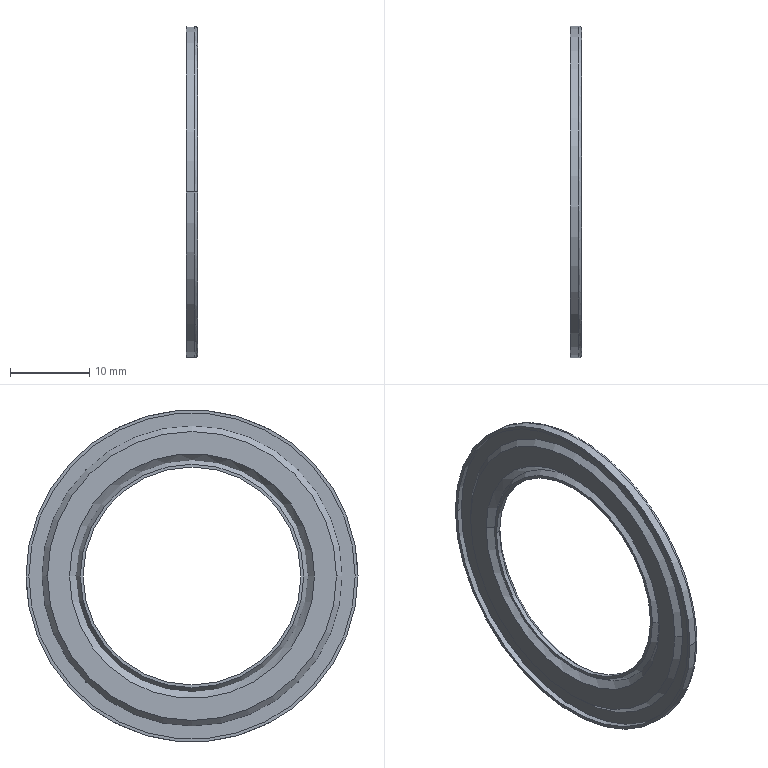Part | STEP file | Microwave Drying Flat Conveyor-inafag_ucfl204_62o9y6gnj3059x015y4y3bh4_09 | 1 solid | 27 faces | box 1.397 x 42 x 42 mm | volume 599.533 mm3 | cone 12 | plane 7 | cylinder 6 | spline 2 | commonest cylinder face diameters 27.56 x2 41.278 x2 42 x2
STEP:
#1=CARTESIAN_POINT('',(8.679,21.,0.));
#2=VERTEX_POINT('',#1);
#3=CARTESIAN_POINT('',(8.679,-21.,0.));
#4=VERTEX_POINT('',#3);
#5=CARTESIAN_POINT('',(8.679,0.,0.));
#6=DIRECTION('',(-1.,0.,0.));
#7=DIRECTION('',(0.,-1.,0.));
#8=AXIS2_PLACEMENT_3D('',#5,#6,#7);
#9=CIRCLE('',#8,21.);
#10=EDGE_CURVE('',#2,#4,#9,.T.);
#11=ORIENTED_EDGE('',*,*,#10,.F.);
#12=CARTESIAN_POINT('',(9.04,20.639,0.));
#13=VERTEX_POINT('',#12);
#14=CARTESIAN_POINT('',(8.679,20.639,0.));
#15=DIRECTION('',(0.,0.,-1.));
#16=DIRECTION('',(0.,1.,0.));
#17=AXIS2_PLACEMENT_3D('',#14,#15,#16);
#18=CIRCLE('',#17,0.361);
#19=EDGE_CURVE('',#2,#13,#18,.T.);
#20=ORIENTED_EDGE('',*,*,#19,.T.);
#21=CARTESIAN_POINT('',(9.04,-20.639,0.));
#22=VERTEX_POINT('',#21);
#23=CARTESIAN_POINT('',(9.04,20.639,0.));
#24=CARTESIAN_POINT('',(9.04,20.639,-41.278));
#25=CARTESIAN_POINT('',(9.04,-20.639,-41.278));
#26=CARTESIAN_POINT('',(9.04,-20.639,0.));
#27=(BOUNDED_CURVE()B_SPLINE_CURVE(3,(#23,#24,#25,#26),.UNSPECIFIED.,.F.,.F.)B_SPLINE_CURVE_WITH_KNOTS((4,4),(0.25,0.75),.UNSPECIFIED.)CURVE()GEOMETRIC_REPRESENTATION_ITEM()RATIONAL_B_SPLINE_CURVE((1.,0.3333,0.3333,1.))REPRESENTATION_ITEM(''));
#28=EDGE_CURVE('',#13,#22,#27,.T.);
#29=ORIENTED_EDGE('',*,*,#28,.T.);
#30=CARTESIAN_POINT('',(8.679,-20.639,0.));
#31=DIRECTION('',(0.,0.,1.));
#32=DIRECTION('',(0.,-1.,0.));
#33=AXIS2_PLACEMENT_3D('',#30,#31,#32);
#34=CIRCLE('',#33,0.361);
#35=EDGE_CURVE('',#4,#22,#34,.T.);
#36=ORIENTED_EDGE('',*,*,#35,.F.);
#37=EDGE_LOOP('',(#11,#20,#29,#36));
#38=FACE_OUTER_BOUND('',#37,.T.);
#39=CARTESIAN_POINT('',(8.679,21.,0.));
#40=CARTESIAN_POINT('',(8.679,21.,-42.));
#41=CARTESIAN_POINT('',(8.679,-21.,-42.));
#42=CARTESIAN_POINT('',(8.679,-21.,0.));
#43=CARTESIAN_POINT('',(8.89,21.,0.));
#44=CARTESIAN_POINT('',(8.89,21.,-42.));
#45=CARTESIAN_POINT('',(8.89,-21.,-42.));
#46=CARTESIAN_POINT('',(8.89,-21.,0.));
#47=CARTESIAN_POINT('',(9.04,20.85,0.));
#48=CARTESIAN_POINT('',(9.04,20.85,-41.701));
#49=CARTESIAN_POINT('',(9.04,-20.85,-41.701));
#50=CARTESIAN_POINT('',(9.04,-20.85,0.));
#51=CARTESIAN_POINT('',(9.04,20.639,0.));
#52=CARTESIAN_POINT('',(9.04,20.639,-41.278));
#53=CARTESIAN_POINT('',(9.04,-20.639,-41.278));
#54=CARTESIAN_POINT('',(9.04,-20.639,0.));
#55=(BOUNDED_SURFACE()B_SPLINE_SURFACE(3,3,((#39,#40,#41,#42),(#43,#44,#45,#46),(#47,#48,#49,#50),(#51,#52,#53,#54)),.UNSPECIFIED.,.F.,.F.,.F.)B_SPLINE_SURFACE_WITH_KNOTS((4,4),(4,4),(0.,1.),(0.,1.),.UNSPECIFIED.)GEOMETRIC_REPRESENTATION_ITEM()RATIONAL_B_SPLINE_SURFACE(((1.,0.3333,0.3333,1.),(0.8047,0.2682,0.2682,0.8047),(0.8047,0.2682,0.2682,0.8047),(1.,0.3333,0.3333,1.)))REPRESENTATION_ITEM('')SURFACE());
#56=ADVANCED_FACE('',(#38),#55,.T.);
#57=CARTESIAN_POINT('',(7.643,-18.275,0.));
#58=VERTEX_POINT('',#57);
#59=CARTESIAN_POINT('',(7.643,18.275,0.));
#60=VERTEX_POINT('',#59);
#61=CARTESIAN_POINT('',(7.643,0.,0.));
#62=DIRECTION('',(-1.,0.,0.));
#63=DIRECTION('',(0.,1.,0.));
#64=AXIS2_PLACEMENT_3D('',#61,#62,#63);
#65=CIRCLE('',#64,18.275);
#66=EDGE_CURVE('',#58,#60,#65,.T.);
#67=ORIENTED_EDGE('',*,*,#66,.F.);
#68=CARTESIAN_POINT('',(8.341,-18.974,0.));
#69=VERTEX_POINT('',#68);
#70=CARTESIAN_POINT('',(8.342,-18.974,0.));
#71=DIRECTION('',(0.7071,-0.7071,0.));
#72=VECTOR('',#71,1000.);
#73=LINE('',#70,#72);
#74=EDGE_CURVE('',#58,#69,#73,.T.);
#75=ORIENTED_EDGE('',*,*,#74,.T.);
#76=CARTESIAN_POINT('',(8.342,18.974,0.));
#77=VERTEX_POINT('',#76);
#78=CARTESIAN_POINT('',(8.342,0.,0.));
#79=DIRECTION('',(-1.,0.,0.));
#80=DIRECTION('',(0.,1.,0.));
#81=AXIS2_PLACEMENT_3D('',#78,#79,#80);
#82=CIRCLE('',#81,18.974);
#83=EDGE_CURVE('',#69,#77,#82,.T.);
#84=ORIENTED_EDGE('',*,*,#83,.T.);
#85=CARTESIAN_POINT('',(8.342,18.974,0.));
#86=DIRECTION('',(0.7071,0.7071,0.));
#87=VECTOR('',#86,1000.);
#88=LINE('',#85,#87);
#89=EDGE_CURVE('',#60,#77,#88,.T.);
#90=ORIENTED_EDGE('',*,*,#89,.F.);
#91=EDGE_LOOP('',(#67,#75,#84,#90));
#92=FACE_OUTER_BOUND('',#91,.T.);
#93=CARTESIAN_POINT('',(8.342,0.,0.));
#94=DIRECTION('',(1.,0.,0.));
#95=DIRECTION('',(0.,1.,0.));
#96=AXIS2_PLACEMENT_3D('',#93,#94,#95);
#97=CONICAL_SURFACE('',#96,18.974,0.7854);
#98=ADVANCED_FACE('',(#92),#97,.T.);
#99=CARTESIAN_POINT('',(8.481,-14.659,0.));
#100=VERTEX_POINT('',#99);
#101=CARTESIAN_POINT('',(8.481,14.659,0.));
#102=VERTEX_POINT('',#101);
#103=CARTESIAN_POINT('',(8.481,0.,0.));
#104=DIRECTION('',(1.,0.,0.));
#105=DIRECTION('',(0.,0.,1.));
#106=AXIS2_PLACEMENT_3D('',#103,#104,#105);
#107=CIRCLE('',#106,14.659);
#108=EDGE_CURVE('',#100,#102,#107,.T.);
#109=ORIENTED_EDGE('',*,*,#108,.T.);
#110=CARTESIAN_POINT('',(7.643,15.497,0.));
#111=VERTEX_POINT('',#110);
#112=CARTESIAN_POINT('',(8.481,14.659,0.));
#113=DIRECTION('',(-0.7071,0.7071,0.));
#114=VECTOR('',#113,1000.);
#115=LINE('',#112,#114);
#116=EDGE_CURVE('',#102,#111,#115,.T.);
#117=ORIENTED_EDGE('',*,*,#116,.T.);
#118=CARTESIAN_POINT('',(7.643,-15.497,0.));
#119=VERTEX_POINT('',#118);
#120=CARTESIAN_POINT('',(7.643,0.,0.));
#121=DIRECTION('',(1.,0.,0.));
#122=DIRECTION('',(0.,-1.,0.));
#123=AXIS2_PLACEMENT_3D('',#120,#121,#122);
#124=CIRCLE('',#123,15.497);
#125=EDGE_CURVE('',#119,#111,#124,.T.);
#126=ORIENTED_EDGE('',*,*,#125,.F.);
#127=CARTESIAN_POINT('',(8.481,-14.659,0.));
#128=DIRECTION('',(-0.7071,-0.7071,0.));
#129=VECTOR('',#128,1000.);
#130=LINE('',#127,#129);
#131=EDGE_CURVE('',#100,#119,#130,.T.);
#132=ORIENTED_EDGE('',*,*,#131,.F.);
#133=EDGE_LOOP('',(#109,#117,#126,#132));
#134=FACE_OUTER_BOUND('',#133,.T.);
#135=CARTESIAN_POINT('',(8.481,0.,0.));
#136=DIRECTION('',(-1.,0.,0.));
#137=DIRECTION('',(0.,-1.,0.));
#138=AXIS2_PLACEMENT_3D('',#135,#136,#137);
#139=CONICAL_SURFACE('',#138,14.659,0.7854);
#140=ADVANCED_FACE('',(#134),#139,.F.);
#141=CARTESIAN_POINT('',(7.783,14.141,0.));
#142=VERTEX_POINT('',#141);
#143=CARTESIAN_POINT('',(7.783,-14.141,0.));
#144=VERTEX_POINT('',#143);
#145=CARTESIAN_POINT('',(7.783,0.,0.));
#146=DIRECTION('',(1.,0.,0.));
#147=DIRECTION('',(0.,1.,0.));
#148=AXIS2_PLACEMENT_3D('',#145,#146,#147);
#149=CIRCLE('',#148,14.141);
#150=EDGE_CURVE('',#142,#144,#149,.T.);
#151=ORIENTED_EDGE('',*,*,#150,.T.);
#152=CARTESIAN_POINT('',(8.481,-14.659,0.));
#153=DIRECTION('',(0.8032,-0.5957,0.));
#154=VECTOR('',#153,1000.);
#155=LINE('',#152,#154);
#156=EDGE_CURVE('',#144,#100,#155,.T.);
#157=ORIENTED_EDGE('',*,*,#156,.T.);
#158=CARTESIAN_POINT('',(8.481,0.,0.));
#159=DIRECTION('',(1.,0.,0.));
#160=DIRECTION('',(0.,0.,1.));
#161=AXIS2_PLACEMENT_3D('',#158,#159,#160);
#162=CIRCLE('',#161,14.659);
#163=EDGE_CURVE('',#102,#100,#162,.T.);
#164=ORIENTED_EDGE('',*,*,#163,.F.);
#165=CARTESIAN_POINT('',(8.481,14.659,0.));
#166=DIRECTION('',(0.8032,0.5957,0.));
#167=VECTOR('',#166,1000.);
#168=LINE('',#165,#167);
#169=EDGE_CURVE('',#142,#102,#168,.T.);
#170=ORIENTED_EDGE('',*,*,#169,.F.);
#171=EDGE_LOOP('',(#151,#157,#164,#170));
#172=FACE_OUTER_BOUND('',#171,.T.);
#173=CARTESIAN_POINT('',(8.481,0.,0.));
#174=DIRECTION('',(1.,0.,0.));
#175=DIRECTION('',(0.,1.,0.));
#176=AXIS2_PLACEMENT_3D('',#173,#174,#175);
#177=CONICAL_SURFACE('',#176,14.659,0.6381);
#178=ADVANCED_FACE('',(#172),#177,.T.);
#179=CARTESIAN_POINT('',(8.342,20.639,0.));
#180=VERTEX_POINT('',#179);
#181=CARTESIAN_POINT('',(8.341,-20.639,0.));
#182=VERTEX_POINT('',#181);
#183=CARTESIAN_POINT('',(8.341,0.,0.));
#184=DIRECTION('',(-1.,0.,0.));
#185=DIRECTION('',(0.,-1.,0.));
#186=AXIS2_PLACEMENT_3D('',#183,#184,#185);
#187=CIRCLE('',#186,20.639);
#188=EDGE_CURVE('',#180,#182,#187,.T.);
#189=ORIENTED_EDGE('',*,*,#188,.F.);
#190=CARTESIAN_POINT('',(7.643,20.639,0.));
#191=VERTEX_POINT('',#190);
#192=CARTESIAN_POINT('',(8.342,20.639,0.));
#193=DIRECTION('',(-1.,0.,0.));
#194=VECTOR('',#193,1000.);
#195=LINE('',#192,#194);
#196=EDGE_CURVE('',#180,#191,#195,.T.);
#197=ORIENTED_EDGE('',*,*,#196,.T.);
#198=CARTESIAN_POINT('',(7.643,-20.639,0.));
#199=VERTEX_POINT('',#198);
#200=CARTESIAN_POINT('',(7.643,0.,0.));
#201=DIRECTION('',(-1.,0.,0.));
#202=DIRECTION('',(0.,-1.,0.));
#203=AXIS2_PLACEMENT_3D('',#200,#201,#202);
#204=CIRCLE('',#203,20.639);
#205=EDGE_CURVE('',#191,#199,#204,.T.);
#206=ORIENTED_EDGE('',*,*,#205,.T.);
#207=CARTESIAN_POINT('',(8.341,-20.639,0.));
#208=DIRECTION('',(-1.,0.,0.));
#209=VECTOR('',#208,1000.);
#210=LINE('',#207,#209);
#211=EDGE_CURVE('',#182,#199,#210,.T.);
#212=ORIENTED_EDGE('',*,*,#211,.F.);
#213=EDGE_LOOP('',(#189,#197,#206,#212));
#214=FACE_OUTER_BOUND('',#213,.T.);
#215=CARTESIAN_POINT('',(8.341,0.,0.));
#216=DIRECTION('',(-1.,0.,0.));
#217=DIRECTION('',(0.,-1.,0.));
#218=AXIS2_PLACEMENT_3D('',#215,#216,#217);
#219=CYLINDRICAL_SURFACE('',#218,20.639);
#220=ADVANCED_FACE('',(#214),#219,.F.);
#221=CARTESIAN_POINT('',(8.341,-13.78,0.));
#222=VERTEX_POINT('',#221);
#223=CARTESIAN_POINT('',(8.342,13.78,0.));
#224=VERTEX_POINT('',#223);
#225=CARTESIAN_POINT('',(8.341,0.,0.));
#226=DIRECTION('',(1.,0.,0.));
#227=DIRECTION('',(0.,0.,1.));
#228=AXIS2_PLACEMENT_3D('',#225,#226,#227);
#229=CIRCLE('',#228,13.78);
#230=EDGE_CURVE('',#222,#224,#229,.T.);
#231=ORIENTED_EDGE('',*,*,#230,.T.);
#232=CARTESIAN_POINT('',(7.783,13.78,0.));
#233=VERTEX_POINT('',#232);
#234=CARTESIAN_POINT('',(8.342,13.78,0.));
#235=DIRECTION('',(-1.,0.,0.));
#236=VECTOR('',#235,1000.);
#237=LINE('',#234,#236);
#238=EDGE_CURVE('',#224,#233,#237,.T.);
#239=ORIENTED_EDGE('',*,*,#238,.T.);
#240=CARTESIAN_POINT('',(7.783,-13.78,0.));
#241=VERTEX_POINT('',#240);
#242=CARTESIAN_POINT('',(7.783,0.,0.));
#243=DIRECTION('',(1.,0.,0.));
#244=DIRECTION('',(0.,-1.,0.));
#245=AXIS2_PLACEMENT_3D('',#242,#243,#244);
#246=CIRCLE('',#245,13.78);
#247=EDGE_CURVE('',#241,#233,#246,.T.);
#248=ORIENTED_EDGE('',*,*,#247,.F.);
#249=CARTESIAN_POINT('',(8.341,-13.78,0.));
#250=DIRECTION('',(-1.,0.,0.));
#251=VECTOR('',#250,1000.);
#252=LINE('',#249,#251);
#253=EDGE_CURVE('',#222,#241,#252,.T.);
#254=ORIENTED_EDGE('',*,*,#253,.F.);
#255=EDGE_LOOP('',(#231,#239,#248,#254));
#256=FACE_OUTER_BOUND('',#255,.T.);
#257=CARTESIAN_POINT('',(8.341,0.,0.));
#258=DIRECTION('',(-1.,0.,0.));
#259=DIRECTION('',(0.,-1.,0.));
#260=AXIS2_PLACEMENT_3D('',#257,#258,#259);
#261=CYLINDRICAL_SURFACE('',#260,13.78);
#262=ADVANCED_FACE('',(#256),#261,.F.);
#263=CARTESIAN_POINT('',(8.679,0.,0.));
#264=DIRECTION('',(-1.,0.,0.));
#265=DIRECTION('',(0.,-1.,0.));
#266=AXIS2_PLACEMENT_3D('',#263,#264,#265);
#267=CIRCLE('',#266,21.);
#268=EDGE_CURVE('',#4,#2,#267,.T.);
#269=ORIENTED_EDGE('',*,*,#268,.T.);
#270=CARTESIAN_POINT('',(7.643,21.,0.));
#271=VERTEX_POINT('',#270);
#272=CARTESIAN_POINT('',(8.161,21.,0.));
#273=DIRECTION('',(-1.,0.,0.));
#274=VECTOR('',#273,1000.);
#275=LINE('',#272,#274);
#276=EDGE_CURVE('',#2,#271,#275,.T.);
#277=ORIENTED_EDGE('',*,*,#276,.T.);
#278=CARTESIAN_POINT('',(7.643,-21.,0.));
#279=VERTEX_POINT('',#278);
#280=CARTESIAN_POINT('',(7.643,0.,0.));
#281=DIRECTION('',(-1.,0.,0.));
#282=DIRECTION('',(0.,-1.,0.));
#283=AXIS2_PLACEMENT_3D('',#280,#281,#282);
#284=CIRCLE('',#283,21.);
#285=EDGE_CURVE('',#279,#271,#284,.T.);
#286=ORIENTED_EDGE('',*,*,#285,.F.);
#287=CARTESIAN_POINT('',(8.161,-21.,0.));
#288=DIRECTION('',(-1.,0.,0.));
#289=VECTOR('',#288,1000.);
#290=LINE('',#287,#289);
#291=EDGE_CURVE('',#4,#279,#290,.T.);
#292=ORIENTED_EDGE('',*,*,#291,.F.);
#293=EDGE_LOOP('',(#269,#277,#286,#292));
#294=FACE_OUTER_BOUND('',#293,.T.);
#295=CARTESIAN_POINT('',(8.161,0.,0.));
#296=DIRECTION('',(-1.,0.,0.));
#297=DIRECTION('',(0.,-1.,0.));
#298=AXIS2_PLACEMENT_3D('',#295,#296,#297);
#299=CYLINDRICAL_SURFACE('',#298,21.);
#300=ADVANCED_FACE('',(#294),#299,.T.);
#301=ORIENTED_EDGE('',*,*,#230,.F.);
#302=CARTESIAN_POINT('',(9.04,-14.479,0.));
#303=VERTEX_POINT('',#302);
#304=CARTESIAN_POINT('',(8.341,-13.78,0.));
#305=DIRECTION('',(0.7071,-0.7071,0.));
#306=VECTOR('',#305,1000.);
#307=LINE('',#304,#306);
#308=EDGE_CURVE('',#222,#303,#307,.T.);
#309=ORIENTED_EDGE('',*,*,#308,.T.);
#310=CARTESIAN_POINT('',(9.04,14.479,0.));
#311=VERTEX_POINT('',#310);
#312=CARTESIAN_POINT('',(9.04,0.,0.));
#313=DIRECTION('',(1.,0.,0.));
#314=DIRECTION('',(0.,1.,0.));
#315=AXIS2_PLACEMENT_3D('',#312,#313,#314);
#316=CIRCLE('',#315,14.479);
#317=EDGE_CURVE('',#303,#311,#316,.T.);
#318=ORIENTED_EDGE('',*,*,#317,.T.);
#319=CARTESIAN_POINT('',(8.342,13.78,0.));
#320=DIRECTION('',(0.7071,0.7071,0.));
#321=VECTOR('',#320,1000.);
#322=LINE('',#319,#321);
#323=EDGE_CURVE('',#224,#311,#322,.T.);
#324=ORIENTED_EDGE('',*,*,#323,.F.);
#325=EDGE_LOOP('',(#301,#309,#318,#324));
#326=FACE_OUTER_BOUND('',#325,.T.);
#327=CARTESIAN_POINT('',(8.341,0.,0.));
#328=DIRECTION('',(1.,0.,0.));
#329=DIRECTION('',(0.,1.,0.));
#330=AXIS2_PLACEMENT_3D('',#327,#328,#329);
#331=CONICAL_SURFACE('',#330,13.78,0.7854);
#332=ADVANCED_FACE('',(#326),#331,.F.);
#333=CARTESIAN_POINT('',(9.04,14.84,0.));
#334=VERTEX_POINT('',#333);
#335=CARTESIAN_POINT('',(9.04,-14.84,0.));
#336=VERTEX_POINT('',#335);
#337=CARTESIAN_POINT('',(9.04,0.,0.));
#338=DIRECTION('',(1.,0.,0.));
#339=DIRECTION('',(0.,-1.,0.));
#340=AXIS2_PLACEMENT_3D('',#337,#338,#339);
#341=CIRCLE('',#340,14.84);
#342=EDGE_CURVE('',#334,#336,#341,.T.);
#343=ORIENTED_EDGE('',*,*,#342,.F.);
#344=CARTESIAN_POINT('',(8.342,15.538,0.));
#345=VERTEX_POINT('',#344);
#346=CARTESIAN_POINT('',(8.341,15.538,0.));
#347=DIRECTION('',(-0.7071,0.7071,0.));
#348=VECTOR('',#347,1000.);
#349=LINE('',#346,#348);
#350=EDGE_CURVE('',#334,#345,#349,.T.);
#351=ORIENTED_EDGE('',*,*,#350,.T.);
#352=CARTESIAN_POINT('',(8.341,-15.538,0.));
#353=VERTEX_POINT('',#352);
#354=CARTESIAN_POINT('',(8.341,0.,0.));
#355=DIRECTION('',(1.,0.,0.));
#356=DIRECTION('',(0.,-1.,0.));
#357=AXIS2_PLACEMENT_3D('',#354,#355,#356);
#358=CIRCLE('',#357,15.538);
#359=EDGE_CURVE('',#345,#353,#358,.T.);
#360=ORIENTED_EDGE('',*,*,#359,.T.);
#361=CARTESIAN_POINT('',(8.341,-15.538,0.));
#362=DIRECTION('',(-0.7071,-0.7071,0.));
#363=VECTOR('',#362,1000.);
#364=LINE('',#361,#363);
#365=EDGE_CURVE('',#336,#353,#364,.T.);
#366=ORIENTED_EDGE('',*,*,#365,.F.);
#367=EDGE_LOOP('',(#343,#351,#360,#366));
#368=FACE_OUTER_BOUND('',#367,.T.);
#369=CARTESIAN_POINT('',(8.341,0.,0.));
#370=DIRECTION('',(-1.,0.,0.));
#371=DIRECTION('',(0.,-1.,0.));
#372=AXIS2_PLACEMENT_3D('',#369,#370,#371);
#373=CONICAL_SURFACE('',#372,15.538,0.7854);
#374=ADVANCED_FACE('',(#368),#373,.T.);
#375=CARTESIAN_POINT('',(8.342,18.136,0.));
#376=VERTEX_POINT('',#375);
#377=CARTESIAN_POINT('',(8.341,-18.136,0.));
#378=VERTEX_POINT('',#377);
#379=CARTESIAN_POINT('',(8.342,0.,0.));
#380=DIRECTION('',(-1.,0.,0.));
#381=DIRECTION('',(0.,1.,0.));
#382=AXIS2_PLACEMENT_3D('',#379,#380,#381);
#383=CIRCLE('',#382,18.136);
#384=EDGE_CURVE('',#376,#378,#383,.T.);
#385=ORIENTED_EDGE('',*,*,#384,.T.);
#386=CARTESIAN_POINT('',(9.04,-18.834,0.));
#387=VERTEX_POINT('',#386);
#388=CARTESIAN_POINT('',(8.341,-18.136,0.));
#389=DIRECTION('',(0.7071,-0.7071,0.));
#390=VECTOR('',#389,1000.);
#391=LINE('',#388,#390);
#392=EDGE_CURVE('',#378,#387,#391,.T.);
#393=ORIENTED_EDGE('',*,*,#392,.T.);
#394=CARTESIAN_POINT('',(9.04,18.834,0.));
#395=VERTEX_POINT('',#394);
#396=CARTESIAN_POINT('',(9.04,0.,0.));
#397=DIRECTION('',(-1.,0.,0.));
#398=DIRECTION('',(0.,1.,0.));
#399=AXIS2_PLACEMENT_3D('',#396,#397,#398);
#400=CIRCLE('',#399,18.834);
#401=EDGE_CURVE('',#395,#387,#400,.T.);
#402=ORIENTED_EDGE('',*,*,#401,.F.);
#403=CARTESIAN_POINT('',(8.342,18.136,0.));
#404=DIRECTION('',(0.7071,0.7071,0.));
#405=VECTOR('',#404,1000.);
#406=LINE('',#403,#405);
#407=EDGE_CURVE('',#376,#395,#406,.T.);
#408=ORIENTED_EDGE('',*,*,#407,.F.);
#409=EDGE_LOOP('',(#385,#393,#402,#408));
#410=FACE_OUTER_BOUND('',#409,.T.);
#411=CARTESIAN_POINT('',(8.342,0.,0.));
#412=DIRECTION('',(1.,0.,0.));
#413=DIRECTION('',(0.,1.,0.));
#414=AXIS2_PLACEMENT_3D('',#411,#412,#413);
#415=CONICAL_SURFACE('',#414,18.136,0.7854);
#416=ADVANCED_FACE('',(#410),#415,.F.);
#417=CARTESIAN_POINT('',(7.643,0.,0.));
#418=DIRECTION('',(-1.,0.,0.));
#419=DIRECTION('',(0.,1.,0.));
#420=AXIS2_PLACEMENT_3D('',#417,#418,#419);
#421=CIRCLE('',#420,18.275);
#422=EDGE_CURVE('',#60,#58,#421,.T.);
#423=ORIENTED_EDGE('',*,*,#422,.T.);
#424=ORIENTED_EDGE('',*,*,#66,.T.);
#425=EDGE_LOOP('',(#423,#424));
#426=FACE_OUTER_BOUND('',#425,.T.);
#427=ORIENTED_EDGE('',*,*,#125,.T.);
#428=CARTESIAN_POINT('',(7.643,0.,0.));
#429=DIRECTION('',(1.,0.,0.));
#430=DIRECTION('',(0.,-1.,0.));
#431=AXIS2_PLACEMENT_3D('',#428,#429,#430);
#432=CIRCLE('',#431,15.497);
#433=EDGE_CURVE('',#111,#119,#432,.T.);
#434=ORIENTED_EDGE('',*,*,#433,.T.);
#435=EDGE_LOOP('',(#427,#434));
#436=FACE_BOUND('',#435,.T.);
#437=CARTESIAN_POINT('',(7.643,0.,16.886));
#438=DIRECTION('',(-1.,0.,0.));
#439=DIRECTION('',(0.,-1.,0.));
#440=AXIS2_PLACEMENT_3D('',#437,#438,#439);
#441=PLANE('',#440);
#442=ADVANCED_FACE('',(#426,#436),#441,.T.);
#443=ORIENTED_EDGE('',*,*,#74,.F.);
#444=ORIENTED_EDGE('',*,*,#422,.F.);
#445=ORIENTED_EDGE('',*,*,#89,.T.);
#446=CARTESIAN_POINT('',(8.342,0.,0.));
#447=DIRECTION('',(-1.,0.,0.));
#448=DIRECTION('',(0.,1.,0.));
#449=AXIS2_PLACEMENT_3D('',#446,#447,#448);
#450=CIRCLE('',#449,18.974);
#451=EDGE_CURVE('',#77,#69,#450,.T.);
#452=ORIENTED_EDGE('',*,*,#451,.T.);
#453=EDGE_LOOP('',(#443,#444,#445,#452));
#454=FACE_OUTER_BOUND('',#453,.T.);
#455=CARTESIAN_POINT('',(8.342,0.,0.));
#456=DIRECTION('',(1.,0.,0.));
#457=DIRECTION('',(0.,1.,0.));
#458=AXIS2_PLACEMENT_3D('',#455,#456,#457);
#459=CONICAL_SURFACE('',#458,18.974,0.7854);
#460=ADVANCED_FACE('',(#454),#459,.T.);
#461=ORIENTED_EDGE('',*,*,#116,.F.);
#462=ORIENTED_EDGE('',*,*,#163,.T.);
#463=ORIENTED_EDGE('',*,*,#131,.T.);
#464=ORIENTED_EDGE('',*,*,#433,.F.);
#465=EDGE_LOOP('',(#461,#462,#463,#464));
#466=FACE_OUTER_BOUND('',#465,.T.);
#467=CARTESIAN_POINT('',(8.481,0.,0.));
#468=DIRECTION('',(-1.,0.,0.));
#469=DIRECTION('',(0.,-1.,0.));
#470=AXIS2_PLACEMENT_3D('',#467,#468,#469);
#471=CONICAL_SURFACE('',#470,14.659,0.7854);
#472=ADVANCED_FACE('',(#466),#471,.F.);
#473=CARTESIAN_POINT('',(8.341,0.,0.));
#474=DIRECTION('',(-1.,0.,0.));
#475=DIRECTION('',(0.,-1.,0.));
#476=AXIS2_PLACEMENT_3D('',#473,#474,#475);
#477=CIRCLE('',#476,20.639);
#478=EDGE_CURVE('',#182,#180,#477,.T.);
#479=ORIENTED_EDGE('',*,*,#478,.T.);
#480=ORIENTED_EDGE('',*,*,#188,.T.);
#481=EDGE_LOOP('',(#479,#480));
#482=FACE_OUTER_BOUND('',#481,.T.);
#483=ORIENTED_EDGE('',*,*,#451,.F.);
#484=ORIENTED_EDGE('',*,*,#83,.F.);
#485=EDGE_LOOP('',(#483,#484));
#486=FACE_BOUND('',#485,.T.);
#487=CARTESIAN_POINT('',(8.341,0.,19.806));
#488=DIRECTION('',(-1.,0.,0.));
#489=DIRECTION('',(0.,-1.,0.));
#490=AXIS2_PLACEMENT_3D('',#487,#488,#489);
#491=PLANE('',#490);
#492=ADVANCED_FACE('',(#482,#486),#491,.T.);
#493=ORIENTED_EDGE('',*,*,#156,.F.);
#494=CARTESIAN_POINT('',(7.783,0.,0.));
#495=DIRECTION('',(1.,0.,0.));
#496=DIRECTION('',(0.,1.,0.));
#497=AXIS2_PLACEMENT_3D('',#494,#495,#496);
#498=CIRCLE('',#497,14.141);
#499=EDGE_CURVE('',#144,#142,#498,.T.);
#500=ORIENTED_EDGE('',*,*,#499,.T.);
#501=ORIENTED_EDGE('',*,*,#169,.T.);
#502=ORIENTED_EDGE('',*,*,#108,.F.);
#503=EDGE_LOOP('',(#493,#500,#501,#502));
#504=FACE_OUTER_BOUND('',#503,.T.);
#505=CARTESIAN_POINT('',(8.481,0.,0.));
#506=DIRECTION('',(1.,0.,0.));
#507=DIRECTION('',(0.,1.,0.));
#508=AXIS2_PLACEMENT_3D('',#505,#506,#507);
#509=CONICAL_SURFACE('',#508,14.659,0.6381);
#510=ADVANCED_FACE('',(#504),#509,.T.);
#511=ORIENTED_EDGE('',*,*,#196,.F.);
#512=ORIENTED_EDGE('',*,*,#478,.F.);
#513=ORIENTED_EDGE('',*,*,#211,.T.);
#514=CARTESIAN_POINT('',(7.643,0.,0.));
#515=DIRECTION('',(-1.,0.,0.));
#516=DIRECTION('',(0.,-1.,0.));
#517=AXIS2_PLACEMENT_3D('',#514,#515,#516);
#518=CIRCLE('',#517,20.639);
#519=EDGE_CURVE('',#199,#191,#518,.T.);
#520=ORIENTED_EDGE('',*,*,#519,.T.);
#521=EDGE_LOOP('',(#511,#512,#513,#520));
#522=FACE_OUTER_BOUND('',#521,.T.);
#523=CARTESIAN_POINT('',(8.341,0.,0.));
#524=DIRECTION('',(-1.,0.,0.));
#525=DIRECTION('',(0.,-1.,0.));
#526=AXIS2_PLACEMENT_3D('',#523,#524,#525);
#527=CYLINDRICAL_SURFACE('',#526,20.639);
#528=ADVANCED_FACE('',(#522),#527,.F.);
#529=ORIENTED_EDGE('',*,*,#150,.F.);
#530=ORIENTED_EDGE('',*,*,#499,.F.);
#531=EDGE_LOOP('',(#529,#530));
#532=FACE_OUTER_BOUND('',#531,.T.);
#533=ORIENTED_EDGE('',*,*,#247,.T.);
#534=CARTESIAN_POINT('',(7.783,0.,0.));
#535=DIRECTION('',(1.,0.,0.));
#536=DIRECTION('',(0.,-1.,0.));
#537=AXIS2_PLACEMENT_3D('',#534,#535,#536);
#538=CIRCLE('',#537,13.78);
#539=EDGE_CURVE('',#233,#241,#538,.T.);
#540=ORIENTED_EDGE('',*,*,#539,.T.);
#541=EDGE_LOOP('',(#533,#540));
#542=FACE_BOUND('',#541,.T.);
#543=CARTESIAN_POINT('',(7.783,0.,13.961));
#544=DIRECTION('',(-1.,0.,0.));
#545=DIRECTION('',(0.,-1.,0.));
#546=AXIS2_PLACEMENT_3D('',#543,#544,#545);
#547=PLANE('',#546);
#548=ADVANCED_FACE('',(#532,#542),#547,.T.);
#549=ORIENTED_EDGE('',*,*,#285,.T.);
#550=CARTESIAN_POINT('',(7.643,0.,0.));
#551=DIRECTION('',(-1.,0.,0.));
#552=DIRECTION('',(0.,-1.,0.));
#553=AXIS2_PLACEMENT_3D('',#550,#551,#552);
#554=CIRCLE('',#553,21.);
#555=EDGE_CURVE('',#271,#279,#554,.T.);
#556=ORIENTED_EDGE('',*,*,#555,.T.);
#557=EDGE_LOOP('',(#549,#556));
#558=FACE_OUTER_BOUND('',#557,.T.);
#559=ORIENTED_EDGE('',*,*,#519,.F.);
#560=ORIENTED_EDGE('',*,*,#205,.F.);
#561=EDGE_LOOP('',(#559,#560));
#562=FACE_BOUND('',#561,.T.);
#563=CARTESIAN_POINT('',(7.643,0.,20.82));
#564=DIRECTION('',(-1.,0.,0.));
#565=DIRECTION('',(0.,-1.,0.));
#566=AXIS2_PLACEMENT_3D('',#563,#564,#565);
#567=PLANE('',#566);
#568=ADVANCED_FACE('',(#558,#562),#567,.T.);
#569=ORIENTED_EDGE('',*,*,#238,.F.);
#570=CARTESIAN_POINT('',(8.341,0.,0.));
#571=DIRECTION('',(1.,0.,0.));
#572=DIRECTION('',(0.,0.,1.));
#573=AXIS2_PLACEMENT_3D('',#570,#571,#572);
#574=CIRCLE('',#573,13.78);
#575=EDGE_CURVE('',#224,#222,#574,.T.);
#576=ORIENTED_EDGE('',*,*,#575,.T.);
#577=ORIENTED_EDGE('',*,*,#253,.T.);
#578=ORIENTED_EDGE('',*,*,#539,.F.);
#579=EDGE_LOOP('',(#569,#576,#577,#578));
#580=FACE_OUTER_BOUND('',#579,.T.);
#581=CARTESIAN_POINT('',(8.341,0.,0.));
#582=DIRECTION('',(-1.,0.,0.));
#583=DIRECTION('',(0.,-1.,0.));
#584=AXIS2_PLACEMENT_3D('',#581,#582,#583);
#585=CYLINDRICAL_SURFACE('',#584,13.78);
#586=ADVANCED_FACE('',(#580),#585,.F.);
#587=ORIENTED_EDGE('',*,*,#276,.F.);
#588=ORIENTED_EDGE('',*,*,#10,.T.);
#589=ORIENTED_EDGE('',*,*,#291,.T.);
#590=ORIENTED_EDGE('',*,*,#555,.F.);
#591=EDGE_LOOP('',(#587,#588,#589,#590));
#592=FACE_OUTER_BOUND('',#591,.T.);
#593=CARTESIAN_POINT('',(8.161,0.,0.));
#594=DIRECTION('',(-1.,0.,0.));
#595=DIRECTION('',(0.,-1.,0.));
#596=AXIS2_PLACEMENT_3D('',#593,#594,#595);
#597=CYLINDRICAL_SURFACE('',#596,21.);
#598=ADVANCED_FACE('',(#592),#597,.T.);
#599=ORIENTED_EDGE('',*,*,#308,.F.);
#600=ORIENTED_EDGE('',*,*,#575,.F.);
#601=ORIENTED_EDGE('',*,*,#323,.T.);
#602=CARTESIAN_POINT('',(9.04,0.,0.));
#603=DIRECTION('',(1.,0.,0.));
#604=DIRECTION('',(0.,1.,0.));
#605=AXIS2_PLACEMENT_3D('',#602,#603,#604);
#606=CIRCLE('',#605,14.479);
#607=EDGE_CURVE('',#311,#303,#606,.T.);
#608=ORIENTED_EDGE('',*,*,#607,.T.);
#609=EDGE_LOOP('',(#599,#600,#601,#608));
#610=FACE_OUTER_BOUND('',#609,.T.);
#611=CARTESIAN_POINT('',(8.341,0.,0.));
#612=DIRECTION('',(1.,0.,0.));
#613=DIRECTION('',(0.,1.,0.));
#614=AXIS2_PLACEMENT_3D('',#611,#612,#613);
#615=CONICAL_SURFACE('',#614,13.78,0.7854);
#616=ADVANCED_FACE('',(#610),#615,.F.);
#617=ORIENTED_EDGE('',*,*,#19,.F.);
#618=ORIENTED_EDGE('',*,*,#268,.F.);
#619=ORIENTED_EDGE('',*,*,#35,.T.);
#620=CARTESIAN_POINT('',(9.04,-20.639,0.));
#621=CARTESIAN_POINT('',(9.04,-20.639,41.278));
#622=CARTESIAN_POINT('',(9.04,20.639,41.278));
#623=CARTESIAN_POINT('',(9.04,20.639,0.));
#624=(BOUNDED_CURVE()B_SPLINE_CURVE(3,(#620,#621,#622,#623),.UNSPECIFIED.,.F.,.T.)B_SPLINE_CURVE_WITH_KNOTS((4,4),(0.75,1.25),.UNSPECIFIED.)CURVE()GEOMETRIC_REPRESENTATION_ITEM()RATIONAL_B_SPLINE_CURVE((1.,0.3333,0.3333,1.))REPRESENTATION_ITEM(''));
#625=EDGE_CURVE('',#22,#13,#624,.T.);
#626=ORIENTED_EDGE('',*,*,#625,.T.);
#627=EDGE_LOOP('',(#617,#618,#619,#626));
#628=FACE_OUTER_BOUND('',#627,.T.);
#629=CARTESIAN_POINT('',(8.679,-21.,0.));
#630=CARTESIAN_POINT('',(8.679,-21.,42.));
#631=CARTESIAN_POINT('',(8.679,21.,42.));
#632=CARTESIAN_POINT('',(8.679,21.,0.));
#633=CARTESIAN_POINT('',(8.89,-21.,0.));
#634=CARTESIAN_POINT('',(8.89,-21.,42.));
#635=CARTESIAN_POINT('',(8.89,21.,42.));
#636=CARTESIAN_POINT('',(8.89,21.,0.));
#637=CARTESIAN_POINT('',(9.04,-20.85,0.));
#638=CARTESIAN_POINT('',(9.04,-20.85,41.701));
#639=CARTESIAN_POINT('',(9.04,20.85,41.701));
#640=CARTESIAN_POINT('',(9.04,20.85,0.));
#641=CARTESIAN_POINT('',(9.04,-20.639,0.));
#642=CARTESIAN_POINT('',(9.04,-20.639,41.278));
#643=CARTESIAN_POINT('',(9.04,20.639,41.278));
#644=CARTESIAN_POINT('',(9.04,20.639,0.));
#645=(BOUNDED_SURFACE()B_SPLINE_SURFACE(3,3,((#629,#630,#631,#632),(#633,#634,#635,#636),(#637,#638,#639,#640),(#641,#642,#643,#644)),.UNSPECIFIED.,.F.,.F.,.F.)B_SPLINE_SURFACE_WITH_KNOTS((4,4),(4,4),(0.,1.),(0.,1.),.UNSPECIFIED.)GEOMETRIC_REPRESENTATION_ITEM()RATIONAL_B_SPLINE_SURFACE(((1.,0.3333,0.3333,1.),(0.8047,0.2682,0.2682,0.8047),(0.8047,0.2682,0.2682,0.8047),(1.,0.3333,0.3333,1.)))REPRESENTATION_ITEM('')SURFACE());
#646=ADVANCED_FACE('',(#628),#645,.T.);
#647=ORIENTED_EDGE('',*,*,#607,.F.);
#648=ORIENTED_EDGE('',*,*,#317,.F.);
#649=EDGE_LOOP('',(#647,#648));
#650=FACE_BOUND('',#649,.T.);
#651=CARTESIAN_POINT('',(9.04,0.,0.));
#652=DIRECTION('',(1.,0.,0.));
#653=DIRECTION('',(0.,-1.,0.));
#654=AXIS2_PLACEMENT_3D('',#651,#652,#653);
#655=CIRCLE('',#654,14.84);
#656=EDGE_CURVE('',#336,#334,#655,.T.);
#657=ORIENTED_EDGE('',*,*,#656,.T.);
#658=ORIENTED_EDGE('',*,*,#342,.T.);
#659=EDGE_LOOP('',(#657,#658));
#660=FACE_OUTER_BOUND('',#659,.T.);
#661=CARTESIAN_POINT('',(9.04,0.,14.659));
#662=DIRECTION('',(1.,0.,0.));
#663=DIRECTION('',(0.,1.,0.));
#664=AXIS2_PLACEMENT_3D('',#661,#662,#663);
#665=PLANE('',#664);
#666=ADVANCED_FACE('',(#650,#660),#665,.T.);
#667=ORIENTED_EDGE('',*,*,#401,.T.);
#668=CARTESIAN_POINT('',(9.04,0.,0.));
#669=DIRECTION('',(-1.,0.,0.));
#670=DIRECTION('',(0.,1.,0.));
#671=AXIS2_PLACEMENT_3D('',#668,#669,#670);
#672=CIRCLE('',#671,18.834);
#673=EDGE_CURVE('',#387,#395,#672,.T.);
#674=ORIENTED_EDGE('',*,*,#673,.T.);
#675=EDGE_LOOP('',(#667,#674));
#676=FACE_BOUND('',#675,.T.);
#677=ORIENTED_EDGE('',*,*,#625,.F.);
#678=ORIENTED_EDGE('',*,*,#28,.F.);
#679=EDGE_LOOP('',(#677,#678));
#680=FACE_OUTER_BOUND('',#679,.T.);
#681=CARTESIAN_POINT('',(9.04,0.,19.737));
#682=DIRECTION('',(1.,0.,0.));
#683=DIRECTION('',(0.,1.,0.));
#684=AXIS2_PLACEMENT_3D('',#681,#682,#683);
#685=PLANE('',#684);
#686=ADVANCED_FACE('',(#676,#680),#685,.T.);
#687=ORIENTED_EDGE('',*,*,#350,.F.);
#688=ORIENTED_EDGE('',*,*,#656,.F.);
#689=ORIENTED_EDGE('',*,*,#365,.T.);
#690=CARTESIAN_POINT('',(8.341,0.,0.));
#691=DIRECTION('',(1.,0.,0.));
#692=DIRECTION('',(0.,-1.,0.));
#693=AXIS2_PLACEMENT_3D('',#690,#691,#692);
#694=CIRCLE('',#693,15.538);
#695=EDGE_CURVE('',#353,#345,#694,.T.);
#696=ORIENTED_EDGE('',*,*,#695,.T.);
#697=EDGE_LOOP('',(#687,#688,#689,#696));
#698=FACE_OUTER_BOUND('',#697,.T.);
#699=CARTESIAN_POINT('',(8.341,0.,0.));
#700=DIRECTION('',(-1.,0.,0.));
#701=DIRECTION('',(0.,-1.,0.));
#702=AXIS2_PLACEMENT_3D('',#699,#700,#701);
#703=CONICAL_SURFACE('',#702,15.538,0.7854);
#704=ADVANCED_FACE('',(#698),#703,.T.);
#705=ORIENTED_EDGE('',*,*,#392,.F.);
#706=CARTESIAN_POINT('',(8.342,0.,0.));
#707=DIRECTION('',(-1.,0.,0.));
#708=DIRECTION('',(0.,1.,0.));
#709=AXIS2_PLACEMENT_3D('',#706,#707,#708);
#710=CIRCLE('',#709,18.136);
#711=EDGE_CURVE('',#378,#376,#710,.T.);
#712=ORIENTED_EDGE('',*,*,#711,.T.);
#713=ORIENTED_EDGE('',*,*,#407,.T.);
#714=ORIENTED_EDGE('',*,*,#673,.F.);
#715=EDGE_LOOP('',(#705,#712,#713,#714));
#716=FACE_OUTER_BOUND('',#715,.T.);
#717=CARTESIAN_POINT('',(8.342,0.,0.));
#718=DIRECTION('',(1.,0.,0.));
#719=DIRECTION('',(0.,1.,0.));
#720=AXIS2_PLACEMENT_3D('',#717,#718,#719);
#721=CONICAL_SURFACE('',#720,18.136,0.7854);
#722=ADVANCED_FACE('',(#716),#721,.F.);
#723=ORIENTED_EDGE('',*,*,#695,.F.);
#724=ORIENTED_EDGE('',*,*,#359,.F.);
#725=EDGE_LOOP('',(#723,#724));
#726=FACE_BOUND('',#725,.T.);
#727=ORIENTED_EDGE('',*,*,#384,.F.);
#728=ORIENTED_EDGE('',*,*,#711,.F.);
#729=EDGE_LOOP('',(#727,#728));
#730=FACE_OUTER_BOUND('',#729,.T.);
#731=CARTESIAN_POINT('',(8.341,0.,16.837));
#732=DIRECTION('',(1.,0.,0.));
#733=DIRECTION('',(0.,1.,0.));
#734=AXIS2_PLACEMENT_3D('',#731,#732,#733);
#735=PLANE('',#734);
#736=ADVANCED_FACE('',(#726,#730),#735,.T.);
#737=CLOSED_SHELL('',(#56,#98,#140,#178,#220,#262,#300,#332,#374,#416,#442,#460,#472,#492,#510,#528,#548,#568,#586,#598,#616,#646,#666,#686,#704,#722,#736));
#738=MANIFOLD_SOLID_BREP('',#737);
#739=CARTESIAN_POINT('',(0.,0.,0.));
#740=DIRECTION('',(0.,0.,1.));
#741=DIRECTION('',(1.,0.,0.));
#742=AXIS2_PLACEMENT_3D('',#739,#740,#741);
#743=(LENGTH_UNIT()NAMED_UNIT(*)SI_UNIT(.MILLI.,.METRE.));
#744=UNCERTAINTY_MEASURE_WITH_UNIT(LENGTH_MEASURE(0.00001),#743,'','');
#745=(NAMED_UNIT(*)PLANE_ANGLE_UNIT()SI_UNIT($,.RADIAN.));
#746=(NAMED_UNIT(*)SI_UNIT($,.STERADIAN.)SOLID_ANGLE_UNIT());
#747=(GEOMETRIC_REPRESENTATION_CONTEXT(3)GLOBAL_UNCERTAINTY_ASSIGNED_CONTEXT((#744))GLOBAL_UNIT_ASSIGNED_CONTEXT((#743,#745,#746))REPRESENTATION_CONTEXT('',''));
#748=ADVANCED_BREP_SHAPE_REPRESENTATION('',(#738,#742),#747);